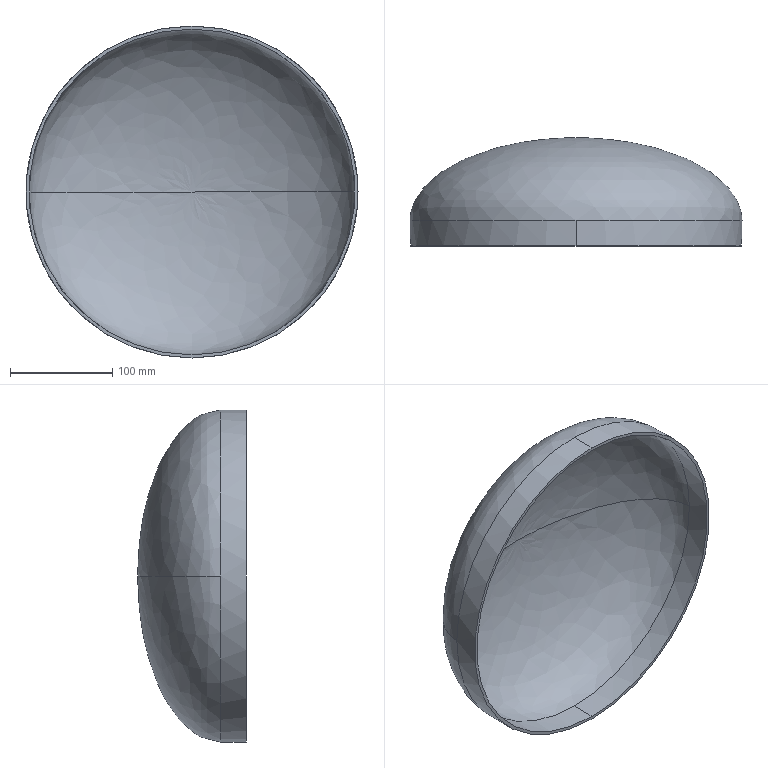Part | SolidWorks | features Revolution 2 | 1 solid | 9 faces | box 325 x 106 x 325 mm | volume 399345 mm3 | spline 4 | cylinder 4 | plane 1 | commonest cylinder face diameters 319 x2 325 x2
STEP:
#1=CARTESIAN_POINT('',(0.,0.,159.5));
#2=VERTEX_POINT('',#1);
#3=CARTESIAN_POINT('',(-159.5,0.,0.));
#4=VERTEX_POINT('',#3);
#5=CARTESIAN_POINT('',(0.,0.,0.));
#6=DIRECTION('',(0.,-1.,0.));
#7=DIRECTION('',(0.,0.,-1.));
#8=AXIS2_PLACEMENT_3D('',#5,#6,#7);
#9=CIRCLE('',#8,159.5);
#10=EDGE_CURVE('',#2,#4,#9,.T.);
#11=ORIENTED_EDGE('',*,*,#10,.T.);
#12=CARTESIAN_POINT('',(0.,78.25,0.));
#13=VERTEX_POINT('',#12);
#14=CARTESIAN_POINT('',(-159.5,0.,0.));
#15=CARTESIAN_POINT('',(-159.5,45.838,0.));
#16=CARTESIAN_POINT('',(-93.433,78.25,0.));
#17=CARTESIAN_POINT('',(0.,78.25,0.));
#18=(BOUNDED_CURVE()B_SPLINE_CURVE(3,(#14,#15,#16,#17),.UNSPECIFIED.,.F.,.F.)B_SPLINE_CURVE_WITH_KNOTS((4,4),(3.142,4.712),.UNSPECIFIED.)CURVE()GEOMETRIC_REPRESENTATION_ITEM()RATIONAL_B_SPLINE_CURVE((1.,0.8047,0.8047,1.))REPRESENTATION_ITEM(''));
#19=EDGE_CURVE('',#4,#13,#18,.T.);
#20=ORIENTED_EDGE('',*,*,#19,.T.);
#21=CARTESIAN_POINT('',(159.5,0.,0.));
#22=VERTEX_POINT('',#21);
#23=CARTESIAN_POINT('',(159.5,0.,0.));
#24=CARTESIAN_POINT('',(159.5,45.838,0.));
#25=CARTESIAN_POINT('',(93.433,78.25,0.));
#26=CARTESIAN_POINT('',(0.,78.25,0.));
#27=(BOUNDED_CURVE()B_SPLINE_CURVE(3,(#23,#24,#25,#26),.UNSPECIFIED.,.F.,.F.)B_SPLINE_CURVE_WITH_KNOTS((4,4),(3.142,4.712),.UNSPECIFIED.)CURVE()GEOMETRIC_REPRESENTATION_ITEM()RATIONAL_B_SPLINE_CURVE((1.,0.8047,0.8047,1.))REPRESENTATION_ITEM(''));
#28=EDGE_CURVE('',#22,#13,#27,.T.);
#29=ORIENTED_EDGE('',*,*,#28,.F.);
#30=CARTESIAN_POINT('',(0.,0.,0.));
#31=DIRECTION('',(0.,-1.,0.));
#32=DIRECTION('',(0.,0.,-1.));
#33=AXIS2_PLACEMENT_3D('',#30,#31,#32);
#34=CIRCLE('',#33,159.5);
#35=EDGE_CURVE('',#22,#2,#34,.T.);
#36=ORIENTED_EDGE('',*,*,#35,.T.);
#37=EDGE_LOOP('',(#11,#20,#29,#36));
#38=FACE_OUTER_BOUND('',#37,.T.);
#39=CARTESIAN_POINT('',(159.5,0.,0.));
#40=CARTESIAN_POINT('',(159.5,0.,319.));
#41=CARTESIAN_POINT('',(-159.5,0.,319.));
#42=CARTESIAN_POINT('',(-159.5,0.,0.));
#43=CARTESIAN_POINT('',(159.5,45.838,0.));
#44=CARTESIAN_POINT('',(159.5,45.838,319.));
#45=CARTESIAN_POINT('',(-159.5,45.838,319.));
#46=CARTESIAN_POINT('',(-159.5,45.838,0.));
#47=CARTESIAN_POINT('',(93.433,78.25,0.));
#48=CARTESIAN_POINT('',(93.433,78.25,186.866));
#49=CARTESIAN_POINT('',(-93.433,78.25,186.866));
#50=CARTESIAN_POINT('',(-93.433,78.25,0.));
#51=CARTESIAN_POINT('',(0.,78.25,0.));
#52=CARTESIAN_POINT('',(0.,78.25,0.));
#53=CARTESIAN_POINT('',(0.,78.25,0.));
#54=CARTESIAN_POINT('',(0.,78.25,0.));
#55=(BOUNDED_SURFACE()B_SPLINE_SURFACE(3,3,((#39,#40,#41,#42),(#43,#44,#45,#46),(#47,#48,#49,#50),(#51,#52,#53,#54)),.UNSPECIFIED.,.F.,.F.,.F.)B_SPLINE_SURFACE_WITH_KNOTS((4,4),(4,4),(0.,1.),(0.,1.),.UNSPECIFIED.)GEOMETRIC_REPRESENTATION_ITEM()RATIONAL_B_SPLINE_SURFACE(((1.,0.3333,0.3333,1.),(0.8047,0.2682,0.2682,0.8047),(0.8047,0.2682,0.2682,0.8047),(1.,0.3333,0.3333,1.)))REPRESENTATION_ITEM('')SURFACE());
#56=ADVANCED_FACE('',(#38),#55,.F.);
#57=CARTESIAN_POINT('',(0.,81.25,0.));
#58=VERTEX_POINT('',#57);
#59=CARTESIAN_POINT('',(162.5,0.,0.));
#60=VERTEX_POINT('',#59);
#61=CARTESIAN_POINT('',(0.,81.25,0.));
#62=CARTESIAN_POINT('',(95.19,81.25,0.));
#63=CARTESIAN_POINT('',(162.5,47.595,0.));
#64=CARTESIAN_POINT('',(162.5,0.,0.));
#65=(BOUNDED_CURVE()B_SPLINE_CURVE(3,(#61,#62,#63,#64),.UNSPECIFIED.,.F.,.F.)B_SPLINE_CURVE_WITH_KNOTS((4,4),(1.571,3.142),.UNSPECIFIED.)CURVE()GEOMETRIC_REPRESENTATION_ITEM()RATIONAL_B_SPLINE_CURVE((1.,0.8047,0.8047,1.))REPRESENTATION_ITEM(''));
#66=EDGE_CURVE('',#58,#60,#65,.T.);
#67=ORIENTED_EDGE('',*,*,#66,.F.);
#68=CARTESIAN_POINT('',(-162.5,0.,0.));
#69=VERTEX_POINT('',#68);
#70=CARTESIAN_POINT('',(0.,81.25,0.));
#71=CARTESIAN_POINT('',(-95.19,81.25,0.));
#72=CARTESIAN_POINT('',(-162.5,47.595,0.));
#73=CARTESIAN_POINT('',(-162.5,0.,0.));
#74=(BOUNDED_CURVE()B_SPLINE_CURVE(3,(#70,#71,#72,#73),.UNSPECIFIED.,.F.,.F.)B_SPLINE_CURVE_WITH_KNOTS((4,4),(1.571,3.142),.UNSPECIFIED.)CURVE()GEOMETRIC_REPRESENTATION_ITEM()RATIONAL_B_SPLINE_CURVE((1.,0.8047,0.8047,1.))REPRESENTATION_ITEM(''));
#75=EDGE_CURVE('',#58,#69,#74,.T.);
#76=ORIENTED_EDGE('',*,*,#75,.T.);
#77=CARTESIAN_POINT('',(0.,0.,162.5));
#78=VERTEX_POINT('',#77);
#79=CARTESIAN_POINT('',(0.,0.,0.));
#80=DIRECTION('',(0.,-1.,0.));
#81=DIRECTION('',(0.,0.,-1.));
#82=AXIS2_PLACEMENT_3D('',#79,#80,#81);
#83=CIRCLE('',#82,162.5);
#84=EDGE_CURVE('',#78,#69,#83,.T.);
#85=ORIENTED_EDGE('',*,*,#84,.F.);
#86=CARTESIAN_POINT('',(0.,0.,0.));
#87=DIRECTION('',(0.,-1.,0.));
#88=DIRECTION('',(0.,0.,-1.));
#89=AXIS2_PLACEMENT_3D('',#86,#87,#88);
#90=CIRCLE('',#89,162.5);
#91=EDGE_CURVE('',#60,#78,#90,.T.);
#92=ORIENTED_EDGE('',*,*,#91,.F.);
#93=EDGE_LOOP('',(#67,#76,#85,#92));
#94=FACE_OUTER_BOUND('',#93,.T.);
#95=CARTESIAN_POINT('',(0.,81.25,0.));
#96=CARTESIAN_POINT('',(0.,81.25,0.));
#97=CARTESIAN_POINT('',(0.,81.25,0.));
#98=CARTESIAN_POINT('',(0.,81.25,0.));
#99=CARTESIAN_POINT('',(95.19,81.25,0.));
#100=CARTESIAN_POINT('',(95.19,81.25,190.381));
#101=CARTESIAN_POINT('',(-95.19,81.25,190.381));
#102=CARTESIAN_POINT('',(-95.19,81.25,0.));
#103=CARTESIAN_POINT('',(162.5,47.595,0.));
#104=CARTESIAN_POINT('',(162.5,47.595,325.));
#105=CARTESIAN_POINT('',(-162.5,47.595,325.));
#106=CARTESIAN_POINT('',(-162.5,47.595,0.));
#107=CARTESIAN_POINT('',(162.5,0.,0.));
#108=CARTESIAN_POINT('',(162.5,0.,325.));
#109=CARTESIAN_POINT('',(-162.5,0.,325.));
#110=CARTESIAN_POINT('',(-162.5,0.,0.));
#111=(BOUNDED_SURFACE()B_SPLINE_SURFACE(3,3,((#95,#96,#97,#98),(#99,#100,#101,#102),(#103,#104,#105,#106),(#107,#108,#109,#110)),.UNSPECIFIED.,.F.,.F.,.F.)B_SPLINE_SURFACE_WITH_KNOTS((4,4),(4,4),(0.,1.),(0.,1.),.UNSPECIFIED.)GEOMETRIC_REPRESENTATION_ITEM()RATIONAL_B_SPLINE_SURFACE(((1.,0.3333,0.3333,1.),(0.8047,0.2682,0.2682,0.8047),(0.8047,0.2682,0.2682,0.8047),(1.,0.3333,0.3333,1.)))REPRESENTATION_ITEM('')SURFACE());
#112=ADVANCED_FACE('',(#94),#111,.F.);
#113=ORIENTED_EDGE('',*,*,#10,.F.);
#114=CARTESIAN_POINT('',(0.,-24.75,159.5));
#115=VERTEX_POINT('',#114);
#116=CARTESIAN_POINT('',(0.,0.,159.5));
#117=DIRECTION('',(0.,-1.,0.));
#118=VECTOR('',#117,1000.);
#119=LINE('',#116,#118);
#120=EDGE_CURVE('',#2,#115,#119,.T.);
#121=ORIENTED_EDGE('',*,*,#120,.T.);
#122=CARTESIAN_POINT('',(0.,-24.75,-159.5));
#123=VERTEX_POINT('',#122);
#124=CARTESIAN_POINT('',(0.,-24.75,0.));
#125=DIRECTION('',(0.,-1.,0.));
#126=DIRECTION('',(0.,0.,-1.));
#127=AXIS2_PLACEMENT_3D('',#124,#125,#126);
#128=CIRCLE('',#127,159.5);
#129=EDGE_CURVE('',#115,#123,#128,.T.);
#130=ORIENTED_EDGE('',*,*,#129,.T.);
#131=CARTESIAN_POINT('',(0.,0.,-159.5));
#132=VERTEX_POINT('',#131);
#133=CARTESIAN_POINT('',(0.,0.,-159.5));
#134=DIRECTION('',(0.,-1.,0.));
#135=VECTOR('',#134,1000.);
#136=LINE('',#133,#135);
#137=EDGE_CURVE('',#132,#123,#136,.T.);
#138=ORIENTED_EDGE('',*,*,#137,.F.);
#139=CARTESIAN_POINT('',(0.,0.,0.));
#140=DIRECTION('',(0.,-1.,0.));
#141=DIRECTION('',(0.,0.,-1.));
#142=AXIS2_PLACEMENT_3D('',#139,#140,#141);
#143=CIRCLE('',#142,159.5);
#144=EDGE_CURVE('',#4,#132,#143,.T.);
#145=ORIENTED_EDGE('',*,*,#144,.F.);
#146=EDGE_LOOP('',(#113,#121,#130,#138,#145));
#147=FACE_OUTER_BOUND('',#146,.T.);
#148=CARTESIAN_POINT('',(0.,0.,0.));
#149=DIRECTION('',(0.,-1.,0.));
#150=DIRECTION('',(0.,0.,-1.));
#151=AXIS2_PLACEMENT_3D('',#148,#149,#150);
#152=CYLINDRICAL_SURFACE('',#151,159.5);
#153=ADVANCED_FACE('',(#147),#152,.F.);
#154=CARTESIAN_POINT('',(0.,0.,-162.5));
#155=VERTEX_POINT('',#154);
#156=CARTESIAN_POINT('',(0.,0.,0.));
#157=DIRECTION('',(0.,-1.,0.));
#158=DIRECTION('',(0.,0.,-1.));
#159=AXIS2_PLACEMENT_3D('',#156,#157,#158);
#160=CIRCLE('',#159,162.5);
#161=EDGE_CURVE('',#155,#60,#160,.T.);
#162=ORIENTED_EDGE('',*,*,#161,.T.);
#163=ORIENTED_EDGE('',*,*,#91,.T.);
#164=CARTESIAN_POINT('',(0.,-24.75,162.5));
#165=VERTEX_POINT('',#164);
#166=CARTESIAN_POINT('',(0.,0.,162.5));
#167=DIRECTION('',(0.,-1.,0.));
#168=VECTOR('',#167,1000.);
#169=LINE('',#166,#168);
#170=EDGE_CURVE('',#78,#165,#169,.T.);
#171=ORIENTED_EDGE('',*,*,#170,.T.);
#172=CARTESIAN_POINT('',(0.,-24.75,-162.5));
#173=VERTEX_POINT('',#172);
#174=CARTESIAN_POINT('',(0.,-24.75,0.));
#175=DIRECTION('',(0.,-1.,0.));
#176=DIRECTION('',(0.,0.,-1.));
#177=AXIS2_PLACEMENT_3D('',#174,#175,#176);
#178=CIRCLE('',#177,162.5);
#179=EDGE_CURVE('',#173,#165,#178,.T.);
#180=ORIENTED_EDGE('',*,*,#179,.F.);
#181=CARTESIAN_POINT('',(0.,0.,-162.5));
#182=DIRECTION('',(0.,-1.,0.));
#183=VECTOR('',#182,1000.);
#184=LINE('',#181,#183);
#185=EDGE_CURVE('',#155,#173,#184,.T.);
#186=ORIENTED_EDGE('',*,*,#185,.F.);
#187=EDGE_LOOP('',(#162,#163,#171,#180,#186));
#188=FACE_OUTER_BOUND('',#187,.T.);
#189=CARTESIAN_POINT('',(0.,0.,0.));
#190=DIRECTION('',(0.,-1.,0.));
#191=DIRECTION('',(0.,0.,-1.));
#192=AXIS2_PLACEMENT_3D('',#189,#190,#191);
#193=CYLINDRICAL_SURFACE('',#192,162.5);
#194=ADVANCED_FACE('',(#188),#193,.T.);
#195=ORIENTED_EDGE('',*,*,#75,.F.);
#196=ORIENTED_EDGE('',*,*,#66,.T.);
#197=ORIENTED_EDGE('',*,*,#161,.F.);
#198=CARTESIAN_POINT('',(0.,0.,0.));
#199=DIRECTION('',(0.,-1.,0.));
#200=DIRECTION('',(0.,0.,-1.));
#201=AXIS2_PLACEMENT_3D('',#198,#199,#200);
#202=CIRCLE('',#201,162.5);
#203=EDGE_CURVE('',#69,#155,#202,.T.);
#204=ORIENTED_EDGE('',*,*,#203,.F.);
#205=EDGE_LOOP('',(#195,#196,#197,#204));
#206=FACE_OUTER_BOUND('',#205,.T.);
#207=CARTESIAN_POINT('',(0.,81.25,0.));
#208=CARTESIAN_POINT('',(0.,81.25,0.));
#209=CARTESIAN_POINT('',(0.,81.25,0.));
#210=CARTESIAN_POINT('',(0.,81.25,0.));
#211=CARTESIAN_POINT('',(-95.19,81.25,0.));
#212=CARTESIAN_POINT('',(-95.19,81.25,-190.381));
#213=CARTESIAN_POINT('',(95.19,81.25,-190.381));
#214=CARTESIAN_POINT('',(95.19,81.25,0.));
#215=CARTESIAN_POINT('',(-162.5,47.595,0.));
#216=CARTESIAN_POINT('',(-162.5,47.595,-325.));
#217=CARTESIAN_POINT('',(162.5,47.595,-325.));
#218=CARTESIAN_POINT('',(162.5,47.595,0.));
#219=CARTESIAN_POINT('',(-162.5,0.,0.));
#220=CARTESIAN_POINT('',(-162.5,0.,-325.));
#221=CARTESIAN_POINT('',(162.5,0.,-325.));
#222=CARTESIAN_POINT('',(162.5,0.,0.));
#223=(BOUNDED_SURFACE()B_SPLINE_SURFACE(3,3,((#207,#208,#209,#210),(#211,#212,#213,#214),(#215,#216,#217,#218),(#219,#220,#221,#222)),.UNSPECIFIED.,.F.,.F.,.F.)B_SPLINE_SURFACE_WITH_KNOTS((4,4),(4,4),(0.,1.),(0.,1.),.UNSPECIFIED.)GEOMETRIC_REPRESENTATION_ITEM()RATIONAL_B_SPLINE_SURFACE(((1.,0.3333,0.3333,1.),(0.8047,0.2682,0.2682,0.8047),(0.8047,0.2682,0.2682,0.8047),(1.,0.3333,0.3333,1.)))REPRESENTATION_ITEM('')SURFACE());
#224=ADVANCED_FACE('',(#206),#223,.F.);
#225=ORIENTED_EDGE('',*,*,#170,.F.);
#226=ORIENTED_EDGE('',*,*,#84,.T.);
#227=ORIENTED_EDGE('',*,*,#203,.T.);
#228=ORIENTED_EDGE('',*,*,#185,.T.);
#229=CARTESIAN_POINT('',(0.,-24.75,0.));
#230=DIRECTION('',(0.,-1.,0.));
#231=DIRECTION('',(0.,0.,-1.));
#232=AXIS2_PLACEMENT_3D('',#229,#230,#231);
#233=CIRCLE('',#232,162.5);
#234=EDGE_CURVE('',#165,#173,#233,.T.);
#235=ORIENTED_EDGE('',*,*,#234,.F.);
#236=EDGE_LOOP('',(#225,#226,#227,#228,#235));
#237=FACE_OUTER_BOUND('',#236,.T.);
#238=CARTESIAN_POINT('',(0.,0.,0.));
#239=DIRECTION('',(0.,-1.,0.));
#240=DIRECTION('',(0.,0.,-1.));
#241=AXIS2_PLACEMENT_3D('',#238,#239,#240);
#242=CYLINDRICAL_SURFACE('',#241,162.5);
#243=ADVANCED_FACE('',(#237),#242,.T.);
#244=CARTESIAN_POINT('',(0.,-24.75,0.));
#245=DIRECTION('',(0.,-1.,0.));
#246=DIRECTION('',(0.,0.,-1.));
#247=AXIS2_PLACEMENT_3D('',#244,#245,#246);
#248=CIRCLE('',#247,159.5);
#249=EDGE_CURVE('',#123,#115,#248,.T.);
#250=ORIENTED_EDGE('',*,*,#249,.F.);
#251=ORIENTED_EDGE('',*,*,#129,.F.);
#252=EDGE_LOOP('',(#250,#251));
#253=FACE_BOUND('',#252,.T.);
#254=ORIENTED_EDGE('',*,*,#179,.T.);
#255=ORIENTED_EDGE('',*,*,#234,.T.);
#256=EDGE_LOOP('',(#254,#255));
#257=FACE_OUTER_BOUND('',#256,.T.);
#258=CARTESIAN_POINT('',(162.5,-24.75,0.));
#259=DIRECTION('',(0.,1.,0.));
#260=DIRECTION('',(0.,0.,1.));
#261=AXIS2_PLACEMENT_3D('',#258,#259,#260);
#262=PLANE('',#261);
#263=ADVANCED_FACE('',(#253,#257),#262,.F.);
#264=ORIENTED_EDGE('',*,*,#120,.F.);
#265=ORIENTED_EDGE('',*,*,#35,.F.);
#266=CARTESIAN_POINT('',(0.,0.,0.));
#267=DIRECTION('',(0.,-1.,0.));
#268=DIRECTION('',(0.,0.,-1.));
#269=AXIS2_PLACEMENT_3D('',#266,#267,#268);
#270=CIRCLE('',#269,159.5);
#271=EDGE_CURVE('',#132,#22,#270,.T.);
#272=ORIENTED_EDGE('',*,*,#271,.F.);
#273=ORIENTED_EDGE('',*,*,#137,.T.);
#274=ORIENTED_EDGE('',*,*,#249,.T.);
#275=EDGE_LOOP('',(#264,#265,#272,#273,#274));
#276=FACE_OUTER_BOUND('',#275,.T.);
#277=CARTESIAN_POINT('',(0.,0.,0.));
#278=DIRECTION('',(0.,-1.,0.));
#279=DIRECTION('',(0.,0.,-1.));
#280=AXIS2_PLACEMENT_3D('',#277,#278,#279);
#281=CYLINDRICAL_SURFACE('',#280,159.5);
#282=ADVANCED_FACE('',(#276),#281,.F.);
#283=ORIENTED_EDGE('',*,*,#19,.F.);
#284=ORIENTED_EDGE('',*,*,#144,.T.);
#285=ORIENTED_EDGE('',*,*,#271,.T.);
#286=ORIENTED_EDGE('',*,*,#28,.T.);
#287=EDGE_LOOP('',(#283,#284,#285,#286));
#288=FACE_OUTER_BOUND('',#287,.T.);
#289=CARTESIAN_POINT('',(-159.5,0.,0.));
#290=CARTESIAN_POINT('',(-159.5,0.,-319.));
#291=CARTESIAN_POINT('',(159.5,0.,-319.));
#292=CARTESIAN_POINT('',(159.5,0.,0.));
#293=CARTESIAN_POINT('',(-159.5,45.838,0.));
#294=CARTESIAN_POINT('',(-159.5,45.838,-319.));
#295=CARTESIAN_POINT('',(159.5,45.838,-319.));
#296=CARTESIAN_POINT('',(159.5,45.838,0.));
#297=CARTESIAN_POINT('',(-93.433,78.25,0.));
#298=CARTESIAN_POINT('',(-93.433,78.25,-186.866));
#299=CARTESIAN_POINT('',(93.433,78.25,-186.866));
#300=CARTESIAN_POINT('',(93.433,78.25,0.));
#301=CARTESIAN_POINT('',(0.,78.25,0.));
#302=CARTESIAN_POINT('',(0.,78.25,0.));
#303=CARTESIAN_POINT('',(0.,78.25,0.));
#304=CARTESIAN_POINT('',(0.,78.25,0.));
#305=(BOUNDED_SURFACE()B_SPLINE_SURFACE(3,3,((#289,#290,#291,#292),(#293,#294,#295,#296),(#297,#298,#299,#300),(#301,#302,#303,#304)),.UNSPECIFIED.,.F.,.F.,.F.)B_SPLINE_SURFACE_WITH_KNOTS((4,4),(4,4),(0.,1.),(0.,1.),.UNSPECIFIED.)GEOMETRIC_REPRESENTATION_ITEM()RATIONAL_B_SPLINE_SURFACE(((1.,0.3333,0.3333,1.),(0.8047,0.2682,0.2682,0.8047),(0.8047,0.2682,0.2682,0.8047),(1.,0.3333,0.3333,1.)))REPRESENTATION_ITEM('')SURFACE());
#306=ADVANCED_FACE('',(#288),#305,.F.);
#307=CLOSED_SHELL('',(#56,#112,#153,#194,#224,#243,#263,#282,#306));
#308=MANIFOLD_SOLID_BREP('',#307);
#309=CARTESIAN_POINT('',(0.,0.,0.));
#310=DIRECTION('',(0.,0.,1.));
#311=DIRECTION('',(1.,0.,0.));
#312=AXIS2_PLACEMENT_3D('',#309,#310,#311);
#313=(LENGTH_UNIT()NAMED_UNIT(*)SI_UNIT(.MILLI.,.METRE.));
#314=UNCERTAINTY_MEASURE_WITH_UNIT(LENGTH_MEASURE(0.00001),#313,'','');
#315=(NAMED_UNIT(*)PLANE_ANGLE_UNIT()SI_UNIT($,.RADIAN.));
#316=(NAMED_UNIT(*)SI_UNIT($,.STERADIAN.)SOLID_ANGLE_UNIT());
#317=(GEOMETRIC_REPRESENTATION_CONTEXT(3)GLOBAL_UNCERTAINTY_ASSIGNED_CONTEXT((#314))GLOBAL_UNIT_ASSIGNED_CONTEXT((#313,#315,#316))REPRESENTATION_CONTEXT('',''));
#318=ADVANCED_BREP_SHAPE_REPRESENTATION('',(#308,#312),#317);